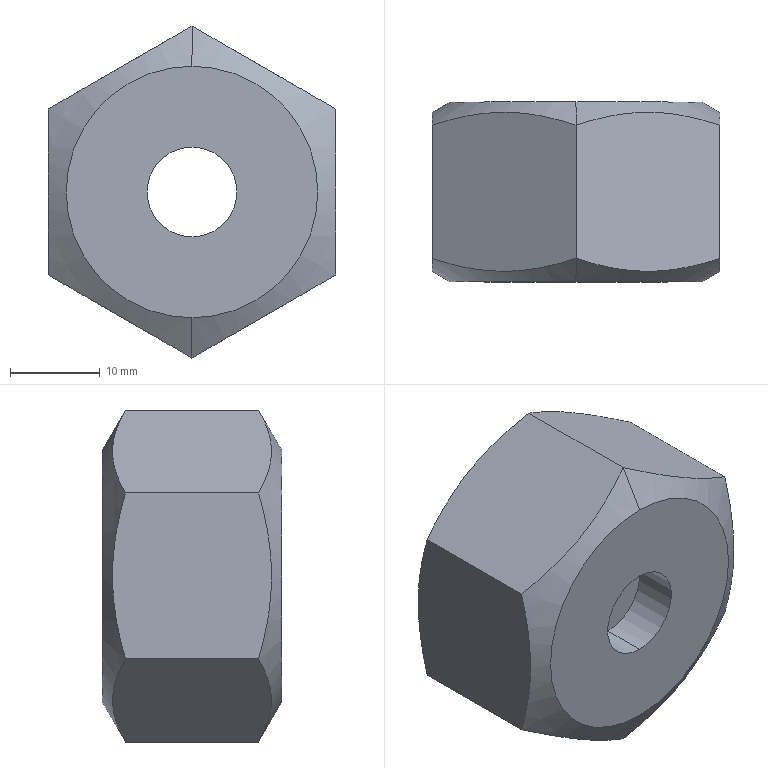Part | SolidWorks | features ICE 2, Extrusion 1, MirrorPattern 1, RevCut 1 | 1 solid | 20 faces | box 32 x 20 x 36.95 mm | volume 13532 mm3 | plane 10 | cylinder 6 | cone 4 | commonest cylinder face diameters 10 x4 28 x2
STEP:
#1=CARTESIAN_POINT('',(0.,-10.,14.));
#2=VERTEX_POINT('',#1);
#3=CARTESIAN_POINT('',(0.,-10.,-14.));
#4=VERTEX_POINT('',#3);
#5=CARTESIAN_POINT('',(0.,-10.,0.));
#6=DIRECTION('',(0.,-1.,0.));
#7=DIRECTION('',(0.,0.,-1.));
#8=AXIS2_PLACEMENT_3D('',#5,#6,#7);
#9=CIRCLE('',#8,14.);
#10=EDGE_CURVE('',#2,#4,#9,.T.);
#11=ORIENTED_EDGE('',*,*,#10,.F.);
#12=CARTESIAN_POINT('',(0.,-7.416,18.475));
#13=VERTEX_POINT('',#12);
#14=CARTESIAN_POINT('',(0.,-10.,14.));
#15=DIRECTION('',(0.,0.5,0.866));
#16=VECTOR('',#15,1000.);
#17=LINE('',#14,#16);
#18=EDGE_CURVE('',#2,#13,#17,.T.);
#19=ORIENTED_EDGE('',*,*,#18,.T.);
#20=CARTESIAN_POINT('',(-16.,-7.416,9.238));
#21=VERTEX_POINT('',#20);
#22=CARTESIAN_POINT('',(-16.,-7.416,9.238));
#23=CARTESIAN_POINT('',(-14.694,-7.852,9.992));
#24=CARTESIAN_POINT('',(-13.378,-8.211,10.751));
#25=CARTESIAN_POINT('',(-10.719,-8.708,12.287));
#26=CARTESIAN_POINT('',(-9.376,-8.844,13.062));
#27=CARTESIAN_POINT('',(-7.335,-8.846,14.24));
#28=CARTESIAN_POINT('',(-6.652,-8.812,14.635));
#29=CARTESIAN_POINT('',(-5.3,-8.682,15.415));
#30=CARTESIAN_POINT('',(-4.629,-8.585,15.803));
#31=CARTESIAN_POINT('',(-2.627,-8.212,16.959));
#32=CARTESIAN_POINT('',(-1.308,-7.852,17.72));
#33=CARTESIAN_POINT('',(0.,-7.416,18.475));
#34=B_SPLINE_CURVE_WITH_KNOTS('',3,(#22,#23,#24,#25,#26,#27,#28,#29,#30,#31,#32,#33),.UNSPECIFIED.,.F.,.F.,(4,2,2,2,2,4),(0.000000238,0.004665,0.00933,0.01166,0.01399,0.01866),.UNSPECIFIED.);
#35=EDGE_CURVE('',#21,#13,#34,.T.);
#36=ORIENTED_EDGE('',*,*,#35,.F.);
#37=CARTESIAN_POINT('',(-16.,-7.416,-9.238));
#38=VERTEX_POINT('',#37);
#39=CARTESIAN_POINT('',(-16.,-7.416,-9.238));
#40=CARTESIAN_POINT('',(-16.,-7.85,-7.733));
#41=CARTESIAN_POINT('',(-16.,-8.209,-6.216));
#42=CARTESIAN_POINT('',(-16.,-8.708,-3.141));
#43=CARTESIAN_POINT('',(-16.,-8.845,-1.584));
#44=CARTESIAN_POINT('',(-16.,-8.845,0.7894));
#45=CARTESIAN_POINT('',(-16.,-8.811,1.576));
#46=CARTESIAN_POINT('',(-16.,-8.68,3.136));
#47=CARTESIAN_POINT('',(-16.,-8.583,3.91));
#48=CARTESIAN_POINT('',(-16.,-8.209,6.217));
#49=CARTESIAN_POINT('',(-16.,-7.85,7.734));
#50=CARTESIAN_POINT('',(-16.,-7.416,9.238));
#51=B_SPLINE_CURVE_WITH_KNOTS('',3,(#39,#40,#41,#42,#43,#44,#45,#46,#47,#48,#49,#50),.UNSPECIFIED.,.F.,.F.,(4,2,2,2,2,4),(0.02027,0.02496,0.02966,0.03201,0.03436,0.03906),.UNSPECIFIED.);
#52=EDGE_CURVE('',#38,#21,#51,.T.);
#53=ORIENTED_EDGE('',*,*,#52,.F.);
#54=CARTESIAN_POINT('',(0.,-7.416,-18.475));
#55=VERTEX_POINT('',#54);
#56=CARTESIAN_POINT('',(0.,-7.416,-18.475));
#57=CARTESIAN_POINT('',(-1.306,-7.852,-17.721));
#58=CARTESIAN_POINT('',(-2.622,-8.211,-16.961));
#59=CARTESIAN_POINT('',(-5.281,-8.708,-15.426));
#60=CARTESIAN_POINT('',(-6.624,-8.844,-14.651));
#61=CARTESIAN_POINT('',(-8.665,-8.846,-13.473));
#62=CARTESIAN_POINT('',(-9.348,-8.812,-13.078));
#63=CARTESIAN_POINT('',(-10.7,-8.682,-12.298));
#64=CARTESIAN_POINT('',(-11.371,-8.585,-11.91));
#65=CARTESIAN_POINT('',(-13.373,-8.212,-10.754));
#66=CARTESIAN_POINT('',(-14.692,-7.852,-9.993));
#67=CARTESIAN_POINT('',(-16.,-7.416,-9.238));
#68=B_SPLINE_CURVE_WITH_KNOTS('',3,(#56,#57,#58,#59,#60,#61,#62,#63,#64,#65,#66,#67),.UNSPECIFIED.,.F.,.F.,(4,2,2,2,2,4),(0.000000238,0.004665,0.00933,0.01166,0.01399,0.01866),.UNSPECIFIED.);
#69=EDGE_CURVE('',#55,#38,#68,.T.);
#70=ORIENTED_EDGE('',*,*,#69,.F.);
#71=CARTESIAN_POINT('',(0.,-10.,-14.));
#72=DIRECTION('',(0.,0.5,-0.866));
#73=VECTOR('',#72,1000.);
#74=LINE('',#71,#73);
#75=EDGE_CURVE('',#4,#55,#74,.T.);
#76=ORIENTED_EDGE('',*,*,#75,.F.);
#77=EDGE_LOOP('',(#11,#19,#36,#53,#70,#76));
#78=FACE_OUTER_BOUND('',#77,.T.);
#79=CARTESIAN_POINT('',(0.,-10.,0.));
#80=DIRECTION('',(0.,1.,0.));
#81=DIRECTION('',(0.,0.,-1.));
#82=AXIS2_PLACEMENT_3D('',#79,#80,#81);
#83=CONICAL_SURFACE('',#82,14.,1.047);
#84=ADVANCED_FACE('',(#78),#83,.T.);
#85=CARTESIAN_POINT('',(0.,10.,-14.));
#86=VERTEX_POINT('',#85);
#87=CARTESIAN_POINT('',(0.,10.,14.));
#88=VERTEX_POINT('',#87);
#89=CARTESIAN_POINT('',(0.,10.,0.));
#90=DIRECTION('',(0.,-1.,0.));
#91=DIRECTION('',(0.,0.,-1.));
#92=AXIS2_PLACEMENT_3D('',#89,#90,#91);
#93=CIRCLE('',#92,14.);
#94=EDGE_CURVE('',#86,#88,#93,.T.);
#95=ORIENTED_EDGE('',*,*,#94,.T.);
#96=CARTESIAN_POINT('',(0.,7.416,18.475));
#97=VERTEX_POINT('',#96);
#98=CARTESIAN_POINT('',(0.,10.,14.));
#99=DIRECTION('',(0.,-0.5,0.866));
#100=VECTOR('',#99,1000.);
#101=LINE('',#98,#100);
#102=EDGE_CURVE('',#88,#97,#101,.T.);
#103=ORIENTED_EDGE('',*,*,#102,.T.);
#104=CARTESIAN_POINT('',(16.,7.416,9.238));
#105=VERTEX_POINT('',#104);
#106=CARTESIAN_POINT('',(16.,7.416,9.238));
#107=CARTESIAN_POINT('',(14.694,7.852,9.992));
#108=CARTESIAN_POINT('',(13.378,8.211,10.751));
#109=CARTESIAN_POINT('',(10.719,8.708,12.287));
#110=CARTESIAN_POINT('',(9.376,8.844,13.062));
#111=CARTESIAN_POINT('',(7.335,8.846,14.24));
#112=CARTESIAN_POINT('',(6.652,8.812,14.635));
#113=CARTESIAN_POINT('',(5.3,8.682,15.415));
#114=CARTESIAN_POINT('',(4.629,8.585,15.803));
#115=CARTESIAN_POINT('',(2.627,8.212,16.959));
#116=CARTESIAN_POINT('',(1.308,7.852,17.72));
#117=CARTESIAN_POINT('',(0.,7.416,18.475));
#118=B_SPLINE_CURVE_WITH_KNOTS('',3,(#106,#107,#108,#109,#110,#111,#112,#113,#114,#115,#116,#117),.UNSPECIFIED.,.F.,.F.,(4,2,2,2,2,4),(0.000000238,0.004665,0.00933,0.01166,0.01399,0.01866),.UNSPECIFIED.);
#119=EDGE_CURVE('',#105,#97,#118,.T.);
#120=ORIENTED_EDGE('',*,*,#119,.F.);
#121=CARTESIAN_POINT('',(16.,7.416,-9.238));
#122=VERTEX_POINT('',#121);
#123=CARTESIAN_POINT('',(16.,7.416,-9.238));
#124=CARTESIAN_POINT('',(16.,7.85,-7.733));
#125=CARTESIAN_POINT('',(16.,8.209,-6.216));
#126=CARTESIAN_POINT('',(16.,8.708,-3.141));
#127=CARTESIAN_POINT('',(16.,8.845,-1.584));
#128=CARTESIAN_POINT('',(16.,8.845,0.7894));
#129=CARTESIAN_POINT('',(16.,8.811,1.576));
#130=CARTESIAN_POINT('',(16.,8.68,3.136));
#131=CARTESIAN_POINT('',(16.,8.583,3.91));
#132=CARTESIAN_POINT('',(16.,8.209,6.217));
#133=CARTESIAN_POINT('',(16.,7.85,7.734));
#134=CARTESIAN_POINT('',(16.,7.416,9.238));
#135=B_SPLINE_CURVE_WITH_KNOTS('',3,(#123,#124,#125,#126,#127,#128,#129,#130,#131,#132,#133,#134),.UNSPECIFIED.,.F.,.F.,(4,2,2,2,2,4),(0.02027,0.02496,0.02966,0.03201,0.03436,0.03906),.UNSPECIFIED.);
#136=EDGE_CURVE('',#122,#105,#135,.T.);
#137=ORIENTED_EDGE('',*,*,#136,.F.);
#138=CARTESIAN_POINT('',(0.,7.416,-18.475));
#139=VERTEX_POINT('',#138);
#140=CARTESIAN_POINT('',(0.,7.416,-18.475));
#141=CARTESIAN_POINT('',(1.306,7.852,-17.721));
#142=CARTESIAN_POINT('',(2.622,8.211,-16.961));
#143=CARTESIAN_POINT('',(5.281,8.708,-15.426));
#144=CARTESIAN_POINT('',(6.624,8.844,-14.651));
#145=CARTESIAN_POINT('',(8.665,8.846,-13.473));
#146=CARTESIAN_POINT('',(9.348,8.812,-13.078));
#147=CARTESIAN_POINT('',(10.7,8.682,-12.298));
#148=CARTESIAN_POINT('',(11.371,8.585,-11.91));
#149=CARTESIAN_POINT('',(13.373,8.212,-10.754));
#150=CARTESIAN_POINT('',(14.692,7.852,-9.993));
#151=CARTESIAN_POINT('',(16.,7.416,-9.238));
#152=B_SPLINE_CURVE_WITH_KNOTS('',3,(#140,#141,#142,#143,#144,#145,#146,#147,#148,#149,#150,#151),.UNSPECIFIED.,.F.,.F.,(4,2,2,2,2,4),(0.000000238,0.004665,0.00933,0.01166,0.01399,0.01866),.UNSPECIFIED.);
#153=EDGE_CURVE('',#139,#122,#152,.T.);
#154=ORIENTED_EDGE('',*,*,#153,.F.);
#155=CARTESIAN_POINT('',(0.,10.,-14.));
#156=DIRECTION('',(0.,-0.5,-0.866));
#157=VECTOR('',#156,1000.);
#158=LINE('',#155,#157);
#159=EDGE_CURVE('',#86,#139,#158,.T.);
#160=ORIENTED_EDGE('',*,*,#159,.F.);
#161=EDGE_LOOP('',(#95,#103,#120,#137,#154,#160));
#162=FACE_OUTER_BOUND('',#161,.T.);
#163=CARTESIAN_POINT('',(0.,10.,0.));
#164=DIRECTION('',(0.,-1.,0.));
#165=DIRECTION('',(0.,0.,-1.));
#166=AXIS2_PLACEMENT_3D('',#163,#164,#165);
#167=CONICAL_SURFACE('',#166,14.,1.047);
#168=ADVANCED_FACE('',(#162),#167,.T.);
#169=CARTESIAN_POINT('',(0.,-1.,-14.));
#170=VERTEX_POINT('',#169);
#171=CARTESIAN_POINT('',(0.,-1.,14.));
#172=VERTEX_POINT('',#171);
#173=CARTESIAN_POINT('',(0.,-1.,0.));
#174=DIRECTION('',(0.,1.,0.));
#175=DIRECTION('',(0.,0.,1.));
#176=AXIS2_PLACEMENT_3D('',#173,#174,#175);
#177=CIRCLE('',#176,14.);
#178=EDGE_CURVE('',#170,#172,#177,.T.);
#179=ORIENTED_EDGE('',*,*,#178,.T.);
#180=CARTESIAN_POINT('',(0.,-5.,14.));
#181=VERTEX_POINT('',#180);
#182=CARTESIAN_POINT('',(0.,-1.,14.));
#183=DIRECTION('',(0.,-1.,0.));
#184=VECTOR('',#183,1000.);
#185=LINE('',#182,#184);
#186=EDGE_CURVE('',#172,#181,#185,.T.);
#187=ORIENTED_EDGE('',*,*,#186,.T.);
#188=CARTESIAN_POINT('',(0.,-5.,-14.));
#189=VERTEX_POINT('',#188);
#190=CARTESIAN_POINT('',(0.,-5.,0.));
#191=DIRECTION('',(0.,1.,0.));
#192=DIRECTION('',(0.,0.,1.));
#193=AXIS2_PLACEMENT_3D('',#190,#191,#192);
#194=CIRCLE('',#193,14.);
#195=EDGE_CURVE('',#189,#181,#194,.T.);
#196=ORIENTED_EDGE('',*,*,#195,.F.);
#197=CARTESIAN_POINT('',(0.,-1.,-14.));
#198=DIRECTION('',(0.,-1.,0.));
#199=VECTOR('',#198,1000.);
#200=LINE('',#197,#199);
#201=EDGE_CURVE('',#170,#189,#200,.T.);
#202=ORIENTED_EDGE('',*,*,#201,.F.);
#203=EDGE_LOOP('',(#179,#187,#196,#202));
#204=FACE_OUTER_BOUND('',#203,.T.);
#205=CARTESIAN_POINT('',(0.,-1.,0.));
#206=DIRECTION('',(0.,-1.,0.));
#207=DIRECTION('',(0.,0.,-1.));
#208=AXIS2_PLACEMENT_3D('',#205,#206,#207);
#209=CYLINDRICAL_SURFACE('',#208,14.);
#210=ADVANCED_FACE('',(#204),#209,.F.);
#211=CARTESIAN_POINT('',(0.,-1.,5.));
#212=VERTEX_POINT('',#211);
#213=CARTESIAN_POINT('',(0.,-1.,-5.));
#214=VERTEX_POINT('',#213);
#215=CARTESIAN_POINT('',(0.,-1.,0.));
#216=DIRECTION('',(0.,-1.,0.));
#217=DIRECTION('',(0.,0.,1.));
#218=AXIS2_PLACEMENT_3D('',#215,#216,#217);
#219=CIRCLE('',#218,5.);
#220=EDGE_CURVE('',#212,#214,#219,.T.);
#221=ORIENTED_EDGE('',*,*,#220,.T.);
#222=CARTESIAN_POINT('',(0.,10.,-5.));
#223=VERTEX_POINT('',#222);
#224=CARTESIAN_POINT('',(0.,-40.,-5.));
#225=DIRECTION('',(0.,1.,0.));
#226=VECTOR('',#225,1000.);
#227=LINE('',#224,#226);
#228=EDGE_CURVE('',#214,#223,#227,.T.);
#229=ORIENTED_EDGE('',*,*,#228,.T.);
#230=CARTESIAN_POINT('',(0.,10.,5.));
#231=VERTEX_POINT('',#230);
#232=CARTESIAN_POINT('',(0.,10.,0.));
#233=DIRECTION('',(0.,1.,0.));
#234=DIRECTION('',(0.,0.,1.));
#235=AXIS2_PLACEMENT_3D('',#232,#233,#234);
#236=CIRCLE('',#235,5.);
#237=EDGE_CURVE('',#223,#231,#236,.T.);
#238=ORIENTED_EDGE('',*,*,#237,.T.);
#239=CARTESIAN_POINT('',(0.,-40.,5.));
#240=DIRECTION('',(0.,1.,0.));
#241=VECTOR('',#240,1000.);
#242=LINE('',#239,#241);
#243=EDGE_CURVE('',#212,#231,#242,.T.);
#244=ORIENTED_EDGE('',*,*,#243,.F.);
#245=EDGE_LOOP('',(#221,#229,#238,#244));
#246=FACE_OUTER_BOUND('',#245,.T.);
#247=CARTESIAN_POINT('',(0.,-40.,0.));
#248=DIRECTION('',(0.,1.,0.));
#249=DIRECTION('',(0.,0.,1.));
#250=AXIS2_PLACEMENT_3D('',#247,#248,#249);
#251=CYLINDRICAL_SURFACE('',#250,5.);
#252=ADVANCED_FACE('',(#246),#251,.F.);
#253=CARTESIAN_POINT('',(0.,-10.,-5.));
#254=VERTEX_POINT('',#253);
#255=CARTESIAN_POINT('',(0.,-10.,5.));
#256=VERTEX_POINT('',#255);
#257=CARTESIAN_POINT('',(0.,-10.,0.));
#258=DIRECTION('',(0.,1.,0.));
#259=DIRECTION('',(0.,0.,1.));
#260=AXIS2_PLACEMENT_3D('',#257,#258,#259);
#261=CIRCLE('',#260,5.);
#262=EDGE_CURVE('',#254,#256,#261,.T.);
#263=ORIENTED_EDGE('',*,*,#262,.F.);
#264=CARTESIAN_POINT('',(0.,-5.,-5.));
#265=VERTEX_POINT('',#264);
#266=CARTESIAN_POINT('',(0.,-40.,-5.));
#267=DIRECTION('',(0.,1.,0.));
#268=VECTOR('',#267,1000.);
#269=LINE('',#266,#268);
#270=EDGE_CURVE('',#254,#265,#269,.T.);
#271=ORIENTED_EDGE('',*,*,#270,.T.);
#272=CARTESIAN_POINT('',(0.,-5.,5.));
#273=VERTEX_POINT('',#272);
#274=CARTESIAN_POINT('',(0.,-5.,0.));
#275=DIRECTION('',(0.,-1.,0.));
#276=DIRECTION('',(0.,0.,1.));
#277=AXIS2_PLACEMENT_3D('',#274,#275,#276);
#278=CIRCLE('',#277,5.);
#279=EDGE_CURVE('',#273,#265,#278,.T.);
#280=ORIENTED_EDGE('',*,*,#279,.F.);
#281=CARTESIAN_POINT('',(0.,-40.,5.));
#282=DIRECTION('',(0.,1.,0.));
#283=VECTOR('',#282,1000.);
#284=LINE('',#281,#283);
#285=EDGE_CURVE('',#256,#273,#284,.T.);
#286=ORIENTED_EDGE('',*,*,#285,.F.);
#287=EDGE_LOOP('',(#263,#271,#280,#286));
#288=FACE_OUTER_BOUND('',#287,.T.);
#289=CARTESIAN_POINT('',(0.,-40.,0.));
#290=DIRECTION('',(0.,1.,0.));
#291=DIRECTION('',(0.,0.,1.));
#292=AXIS2_PLACEMENT_3D('',#289,#290,#291);
#293=CYLINDRICAL_SURFACE('',#292,5.);
#294=ADVANCED_FACE('',(#288),#293,.F.);
#295=ORIENTED_EDGE('',*,*,#270,.F.);
#296=CARTESIAN_POINT('',(0.,-10.,0.));
#297=DIRECTION('',(0.,1.,0.));
#298=DIRECTION('',(0.,0.,1.));
#299=AXIS2_PLACEMENT_3D('',#296,#297,#298);
#300=CIRCLE('',#299,5.);
#301=EDGE_CURVE('',#256,#254,#300,.T.);
#302=ORIENTED_EDGE('',*,*,#301,.F.);
#303=ORIENTED_EDGE('',*,*,#285,.T.);
#304=CARTESIAN_POINT('',(0.,-5.,0.));
#305=DIRECTION('',(0.,-1.,0.));
#306=DIRECTION('',(0.,0.,1.));
#307=AXIS2_PLACEMENT_3D('',#304,#305,#306);
#308=CIRCLE('',#307,5.);
#309=EDGE_CURVE('',#265,#273,#308,.T.);
#310=ORIENTED_EDGE('',*,*,#309,.F.);
#311=EDGE_LOOP('',(#295,#302,#303,#310));
#312=FACE_OUTER_BOUND('',#311,.T.);
#313=CARTESIAN_POINT('',(0.,-40.,0.));
#314=DIRECTION('',(0.,1.,0.));
#315=DIRECTION('',(0.,0.,1.));
#316=AXIS2_PLACEMENT_3D('',#313,#314,#315);
#317=CYLINDRICAL_SURFACE('',#316,5.);
#318=ADVANCED_FACE('',(#312),#317,.F.);
#319=CARTESIAN_POINT('',(16.,-7.416,-9.238));
#320=VERTEX_POINT('',#319);
#321=CARTESIAN_POINT('',(16.,10.,-9.238));
#322=DIRECTION('',(0.,-1.,0.));
#323=VECTOR('',#322,1000.);
#324=LINE('',#321,#323);
#325=EDGE_CURVE('',#122,#320,#324,.T.);
#326=ORIENTED_EDGE('',*,*,#325,.T.);
#327=CARTESIAN_POINT('',(16.,-7.416,-9.238));
#328=CARTESIAN_POINT('',(14.694,-7.852,-9.992));
#329=CARTESIAN_POINT('',(13.378,-8.211,-10.751));
#330=CARTESIAN_POINT('',(10.719,-8.708,-12.287));
#331=CARTESIAN_POINT('',(9.376,-8.844,-13.062));
#332=CARTESIAN_POINT('',(7.335,-8.846,-14.24));
#333=CARTESIAN_POINT('',(6.652,-8.812,-14.635));
#334=CARTESIAN_POINT('',(5.3,-8.682,-15.415));
#335=CARTESIAN_POINT('',(4.629,-8.585,-15.803));
#336=CARTESIAN_POINT('',(2.627,-8.212,-16.959));
#337=CARTESIAN_POINT('',(1.308,-7.852,-17.72));
#338=CARTESIAN_POINT('',(0.,-7.416,-18.475));
#339=B_SPLINE_CURVE_WITH_KNOTS('',3,(#327,#328,#329,#330,#331,#332,#333,#334,#335,#336,#337,#338),.UNSPECIFIED.,.F.,.F.,(4,2,2,2,2,4),(0.000000238,0.004665,0.00933,0.01166,0.01399,0.01866),.UNSPECIFIED.);
#340=EDGE_CURVE('',#320,#55,#339,.T.);
#341=ORIENTED_EDGE('',*,*,#340,.T.);
#342=CARTESIAN_POINT('',(0.,10.,-18.475));
#343=DIRECTION('',(0.,-1.,0.));
#344=VECTOR('',#343,1000.);
#345=LINE('',#342,#344);
#346=EDGE_CURVE('',#139,#55,#345,.T.);
#347=ORIENTED_EDGE('',*,*,#346,.F.);
#348=ORIENTED_EDGE('',*,*,#153,.T.);
#349=EDGE_LOOP('',(#326,#341,#347,#348));
#350=FACE_OUTER_BOUND('',#349,.T.);
#351=CARTESIAN_POINT('',(16.,10.,-9.238));
#352=DIRECTION('',(-0.5,0.,0.866));
#353=DIRECTION('',(0.866,0.,0.5));
#354=AXIS2_PLACEMENT_3D('',#351,#352,#353);
#355=PLANE('',#354);
#356=ADVANCED_FACE('',(#350),#355,.F.);
#357=ORIENTED_EDGE('',*,*,#346,.T.);
#358=ORIENTED_EDGE('',*,*,#69,.T.);
#359=CARTESIAN_POINT('',(-16.,7.416,-9.238));
#360=VERTEX_POINT('',#359);
#361=CARTESIAN_POINT('',(-16.,10.,-9.238));
#362=DIRECTION('',(0.,-1.,0.));
#363=VECTOR('',#362,1000.);
#364=LINE('',#361,#363);
#365=EDGE_CURVE('',#360,#38,#364,.T.);
#366=ORIENTED_EDGE('',*,*,#365,.F.);
#367=CARTESIAN_POINT('',(-16.,7.416,-9.238));
#368=CARTESIAN_POINT('',(-14.694,7.852,-9.992));
#369=CARTESIAN_POINT('',(-13.378,8.211,-10.751));
#370=CARTESIAN_POINT('',(-10.719,8.708,-12.287));
#371=CARTESIAN_POINT('',(-9.376,8.844,-13.062));
#372=CARTESIAN_POINT('',(-7.335,8.846,-14.24));
#373=CARTESIAN_POINT('',(-6.652,8.812,-14.635));
#374=CARTESIAN_POINT('',(-5.3,8.682,-15.415));
#375=CARTESIAN_POINT('',(-4.629,8.585,-15.803));
#376=CARTESIAN_POINT('',(-2.627,8.212,-16.959));
#377=CARTESIAN_POINT('',(-1.308,7.852,-17.72));
#378=CARTESIAN_POINT('',(0.,7.416,-18.475));
#379=B_SPLINE_CURVE_WITH_KNOTS('',3,(#367,#368,#369,#370,#371,#372,#373,#374,#375,#376,#377,#378),.UNSPECIFIED.,.F.,.F.,(4,2,2,2,2,4),(0.000000238,0.004665,0.00933,0.01166,0.01399,0.01866),.UNSPECIFIED.);
#380=EDGE_CURVE('',#360,#139,#379,.T.);
#381=ORIENTED_EDGE('',*,*,#380,.T.);
#382=EDGE_LOOP('',(#357,#358,#366,#381));
#383=FACE_OUTER_BOUND('',#382,.T.);
#384=CARTESIAN_POINT('',(0.,10.,-18.475));
#385=DIRECTION('',(0.5,0.,0.866));
#386=DIRECTION('',(0.866,0.,-0.5));
#387=AXIS2_PLACEMENT_3D('',#384,#385,#386);
#388=PLANE('',#387);
#389=ADVANCED_FACE('',(#383),#388,.F.);
#390=ORIENTED_EDGE('',*,*,#365,.T.);
#391=ORIENTED_EDGE('',*,*,#52,.T.);
#392=CARTESIAN_POINT('',(-16.,7.416,9.238));
#393=VERTEX_POINT('',#392);
#394=CARTESIAN_POINT('',(-16.,10.,9.238));
#395=DIRECTION('',(0.,-1.,0.));
#396=VECTOR('',#395,1000.);
#397=LINE('',#394,#396);
#398=EDGE_CURVE('',#393,#21,#397,.T.);
#399=ORIENTED_EDGE('',*,*,#398,.F.);
#400=CARTESIAN_POINT('',(-16.,7.416,9.238));
#401=CARTESIAN_POINT('',(-16.,7.85,7.733));
#402=CARTESIAN_POINT('',(-16.,8.209,6.216));
#403=CARTESIAN_POINT('',(-16.,8.708,3.141));
#404=CARTESIAN_POINT('',(-16.,8.845,1.584));
#405=CARTESIAN_POINT('',(-16.,8.845,-0.7894));
#406=CARTESIAN_POINT('',(-16.,8.811,-1.576));
#407=CARTESIAN_POINT('',(-16.,8.68,-3.136));
#408=CARTESIAN_POINT('',(-16.,8.583,-3.91));
#409=CARTESIAN_POINT('',(-16.,8.209,-6.217));
#410=CARTESIAN_POINT('',(-16.,7.85,-7.734));
#411=CARTESIAN_POINT('',(-16.,7.416,-9.238));
#412=B_SPLINE_CURVE_WITH_KNOTS('',3,(#400,#401,#402,#403,#404,#405,#406,#407,#408,#409,#410,#411),.UNSPECIFIED.,.F.,.F.,(4,2,2,2,2,4),(0.02027,0.02496,0.02966,0.03201,0.03436,0.03906),.UNSPECIFIED.);
#413=EDGE_CURVE('',#393,#360,#412,.T.);
#414=ORIENTED_EDGE('',*,*,#413,.T.);
#415=EDGE_LOOP('',(#390,#391,#399,#414));
#416=FACE_OUTER_BOUND('',#415,.T.);
#417=CARTESIAN_POINT('',(-16.,10.,-9.238));
#418=DIRECTION('',(1.,0.,0.));
#419=DIRECTION('',(0.,0.,-1.));
#420=AXIS2_PLACEMENT_3D('',#417,#418,#419);
#421=PLANE('',#420);
#422=ADVANCED_FACE('',(#416),#421,.F.);
#423=ORIENTED_EDGE('',*,*,#398,.T.);
#424=ORIENTED_EDGE('',*,*,#35,.T.);
#425=CARTESIAN_POINT('',(0.,10.,18.475));
#426=DIRECTION('',(0.,-1.,0.));
#427=VECTOR('',#426,1000.);
#428=LINE('',#425,#427);
#429=EDGE_CURVE('',#97,#13,#428,.T.);
#430=ORIENTED_EDGE('',*,*,#429,.F.);
#431=CARTESIAN_POINT('',(0.,7.416,18.475));
#432=CARTESIAN_POINT('',(-1.306,7.852,17.721));
#433=CARTESIAN_POINT('',(-2.622,8.211,16.961));
#434=CARTESIAN_POINT('',(-5.281,8.708,15.426));
#435=CARTESIAN_POINT('',(-6.624,8.844,14.651));
#436=CARTESIAN_POINT('',(-8.665,8.846,13.473));
#437=CARTESIAN_POINT('',(-9.348,8.812,13.078));
#438=CARTESIAN_POINT('',(-10.7,8.682,12.298));
#439=CARTESIAN_POINT('',(-11.371,8.585,11.91));
#440=CARTESIAN_POINT('',(-13.373,8.212,10.754));
#441=CARTESIAN_POINT('',(-14.692,7.852,9.993));
#442=CARTESIAN_POINT('',(-16.,7.416,9.238));
#443=B_SPLINE_CURVE_WITH_KNOTS('',3,(#431,#432,#433,#434,#435,#436,#437,#438,#439,#440,#441,#442),.UNSPECIFIED.,.F.,.F.,(4,2,2,2,2,4),(0.000000238,0.004665,0.00933,0.01166,0.01399,0.01866),.UNSPECIFIED.);
#444=EDGE_CURVE('',#97,#393,#443,.T.);
#445=ORIENTED_EDGE('',*,*,#444,.T.);
#446=EDGE_LOOP('',(#423,#424,#430,#445));
#447=FACE_OUTER_BOUND('',#446,.T.);
#448=CARTESIAN_POINT('',(-16.,10.,9.238));
#449=DIRECTION('',(0.5,0.,-0.866));
#450=DIRECTION('',(-0.866,0.,-0.5));
#451=AXIS2_PLACEMENT_3D('',#448,#449,#450);
#452=PLANE('',#451);
#453=ADVANCED_FACE('',(#447),#452,.F.);
#454=ORIENTED_EDGE('',*,*,#429,.T.);
#455=CARTESIAN_POINT('',(16.,-7.416,9.238));
#456=VERTEX_POINT('',#455);
#457=CARTESIAN_POINT('',(0.,-7.416,18.475));
#458=CARTESIAN_POINT('',(1.306,-7.852,17.721));
#459=CARTESIAN_POINT('',(2.622,-8.211,16.961));
#460=CARTESIAN_POINT('',(5.281,-8.708,15.426));
#461=CARTESIAN_POINT('',(6.624,-8.844,14.651));
#462=CARTESIAN_POINT('',(8.665,-8.846,13.473));
#463=CARTESIAN_POINT('',(9.348,-8.812,13.078));
#464=CARTESIAN_POINT('',(10.7,-8.682,12.298));
#465=CARTESIAN_POINT('',(11.371,-8.585,11.91));
#466=CARTESIAN_POINT('',(13.373,-8.212,10.754));
#467=CARTESIAN_POINT('',(14.692,-7.852,9.993));
#468=CARTESIAN_POINT('',(16.,-7.416,9.238));
#469=B_SPLINE_CURVE_WITH_KNOTS('',3,(#457,#458,#459,#460,#461,#462,#463,#464,#465,#466,#467,#468),.UNSPECIFIED.,.F.,.F.,(4,2,2,2,2,4),(0.000000238,0.004665,0.00933,0.01166,0.01399,0.01866),.UNSPECIFIED.);
#470=EDGE_CURVE('',#13,#456,#469,.T.);
#471=ORIENTED_EDGE('',*,*,#470,.T.);
#472=CARTESIAN_POINT('',(16.,10.,9.238));
#473=DIRECTION('',(0.,-1.,0.));
#474=VECTOR('',#473,1000.);
#475=LINE('',#472,#474);
#476=EDGE_CURVE('',#105,#456,#475,.T.);
#477=ORIENTED_EDGE('',*,*,#476,.F.);
#478=ORIENTED_EDGE('',*,*,#119,.T.);
#479=EDGE_LOOP('',(#454,#471,#477,#478));
#480=FACE_OUTER_BOUND('',#479,.T.);
#481=CARTESIAN_POINT('',(0.,10.,18.475));
#482=DIRECTION('',(-0.5,0.,-0.866));
#483=DIRECTION('',(-0.866,0.,0.5));
#484=AXIS2_PLACEMENT_3D('',#481,#482,#483);
#485=PLANE('',#484);
#486=ADVANCED_FACE('',(#480),#485,.F.);
#487=ORIENTED_EDGE('',*,*,#476,.T.);
#488=CARTESIAN_POINT('',(16.,-7.416,9.238));
#489=CARTESIAN_POINT('',(16.,-7.85,7.733));
#490=CARTESIAN_POINT('',(16.,-8.209,6.216));
#491=CARTESIAN_POINT('',(16.,-8.708,3.141));
#492=CARTESIAN_POINT('',(16.,-8.845,1.584));
#493=CARTESIAN_POINT('',(16.,-8.845,-0.7894));
#494=CARTESIAN_POINT('',(16.,-8.811,-1.576));
#495=CARTESIAN_POINT('',(16.,-8.68,-3.136));
#496=CARTESIAN_POINT('',(16.,-8.583,-3.91));
#497=CARTESIAN_POINT('',(16.,-8.209,-6.217));
#498=CARTESIAN_POINT('',(16.,-7.85,-7.734));
#499=CARTESIAN_POINT('',(16.,-7.416,-9.238));
#500=B_SPLINE_CURVE_WITH_KNOTS('',3,(#488,#489,#490,#491,#492,#493,#494,#495,#496,#497,#498,#499),.UNSPECIFIED.,.F.,.F.,(4,2,2,2,2,4),(0.02027,0.02496,0.02966,0.03201,0.03436,0.03906),.UNSPECIFIED.);
#501=EDGE_CURVE('',#456,#320,#500,.T.);
#502=ORIENTED_EDGE('',*,*,#501,.T.);
#503=ORIENTED_EDGE('',*,*,#325,.F.);
#504=ORIENTED_EDGE('',*,*,#136,.T.);
#505=EDGE_LOOP('',(#487,#502,#503,#504));
#506=FACE_OUTER_BOUND('',#505,.T.);
#507=CARTESIAN_POINT('',(16.,10.,9.238));
#508=DIRECTION('',(-1.,0.,0.));
#509=DIRECTION('',(0.,0.,1.));
#510=AXIS2_PLACEMENT_3D('',#507,#508,#509);
#511=PLANE('',#510);
#512=ADVANCED_FACE('',(#506),#511,.F.);
#513=ORIENTED_EDGE('',*,*,#94,.F.);
#514=CARTESIAN_POINT('',(0.,10.,0.));
#515=DIRECTION('',(0.,-1.,0.));
#516=DIRECTION('',(0.,0.,-1.));
#517=AXIS2_PLACEMENT_3D('',#514,#515,#516);
#518=CIRCLE('',#517,14.);
#519=EDGE_CURVE('',#88,#86,#518,.T.);
#520=ORIENTED_EDGE('',*,*,#519,.F.);
#521=EDGE_LOOP('',(#513,#520));
#522=FACE_OUTER_BOUND('',#521,.T.);
#523=CARTESIAN_POINT('',(0.,10.,0.));
#524=DIRECTION('',(0.,1.,0.));
#525=DIRECTION('',(0.,0.,1.));
#526=AXIS2_PLACEMENT_3D('',#523,#524,#525);
#527=CIRCLE('',#526,5.);
#528=EDGE_CURVE('',#231,#223,#527,.T.);
#529=ORIENTED_EDGE('',*,*,#528,.F.);
#530=ORIENTED_EDGE('',*,*,#237,.F.);
#531=EDGE_LOOP('',(#529,#530));
#532=FACE_BOUND('',#531,.T.);
#533=CARTESIAN_POINT('',(0.,10.,0.));
#534=DIRECTION('',(0.,1.,0.));
#535=DIRECTION('',(0.,0.,1.));
#536=AXIS2_PLACEMENT_3D('',#533,#534,#535);
#537=PLANE('',#536);
#538=ADVANCED_FACE('',(#522,#532),#537,.T.);
#539=CARTESIAN_POINT('',(0.,-10.,0.));
#540=DIRECTION('',(0.,-1.,0.));
#541=DIRECTION('',(0.,0.,-1.));
#542=AXIS2_PLACEMENT_3D('',#539,#540,#541);
#543=CIRCLE('',#542,14.);
#544=EDGE_CURVE('',#4,#2,#543,.T.);
#545=ORIENTED_EDGE('',*,*,#544,.T.);
#546=ORIENTED_EDGE('',*,*,#10,.T.);
#547=EDGE_LOOP('',(#545,#546));
#548=FACE_OUTER_BOUND('',#547,.T.);
#549=ORIENTED_EDGE('',*,*,#301,.T.);
#550=ORIENTED_EDGE('',*,*,#262,.T.);
#551=EDGE_LOOP('',(#549,#550));
#552=FACE_BOUND('',#551,.T.);
#553=CARTESIAN_POINT('',(0.,-10.,0.));
#554=DIRECTION('',(0.,1.,0.));
#555=DIRECTION('',(0.,0.,1.));
#556=AXIS2_PLACEMENT_3D('',#553,#554,#555);
#557=PLANE('',#556);
#558=ADVANCED_FACE('',(#548,#552),#557,.F.);
#559=ORIENTED_EDGE('',*,*,#228,.F.);
#560=CARTESIAN_POINT('',(0.,-1.,0.));
#561=DIRECTION('',(0.,-1.,0.));
#562=DIRECTION('',(0.,0.,1.));
#563=AXIS2_PLACEMENT_3D('',#560,#561,#562);
#564=CIRCLE('',#563,5.);
#565=EDGE_CURVE('',#214,#212,#564,.T.);
#566=ORIENTED_EDGE('',*,*,#565,.T.);
#567=ORIENTED_EDGE('',*,*,#243,.T.);
#568=ORIENTED_EDGE('',*,*,#528,.T.);
#569=EDGE_LOOP('',(#559,#566,#567,#568));
#570=FACE_OUTER_BOUND('',#569,.T.);
#571=CARTESIAN_POINT('',(0.,-40.,0.));
#572=DIRECTION('',(0.,1.,0.));
#573=DIRECTION('',(0.,0.,1.));
#574=AXIS2_PLACEMENT_3D('',#571,#572,#573);
#575=CYLINDRICAL_SURFACE('',#574,5.);
#576=ADVANCED_FACE('',(#570),#575,.F.);
#577=ORIENTED_EDGE('',*,*,#178,.F.);
#578=CARTESIAN_POINT('',(0.,-1.,0.));
#579=DIRECTION('',(0.,1.,0.));
#580=DIRECTION('',(0.,0.,1.));
#581=AXIS2_PLACEMENT_3D('',#578,#579,#580);
#582=CIRCLE('',#581,14.);
#583=EDGE_CURVE('',#172,#170,#582,.T.);
#584=ORIENTED_EDGE('',*,*,#583,.F.);
#585=EDGE_LOOP('',(#577,#584));
#586=FACE_OUTER_BOUND('',#585,.T.);
#587=ORIENTED_EDGE('',*,*,#220,.F.);
#588=ORIENTED_EDGE('',*,*,#565,.F.);
#589=EDGE_LOOP('',(#587,#588));
#590=FACE_BOUND('',#589,.T.);
#591=CARTESIAN_POINT('',(0.,-1.,0.));
#592=DIRECTION('',(0.,1.,0.));
#593=DIRECTION('',(0.,0.,1.));
#594=AXIS2_PLACEMENT_3D('',#591,#592,#593);
#595=PLANE('',#594);
#596=ADVANCED_FACE('',(#586,#590),#595,.F.);
#597=ORIENTED_EDGE('',*,*,#195,.T.);
#598=CARTESIAN_POINT('',(0.,-5.,0.));
#599=DIRECTION('',(0.,1.,0.));
#600=DIRECTION('',(0.,0.,1.));
#601=AXIS2_PLACEMENT_3D('',#598,#599,#600);
#602=CIRCLE('',#601,14.);
#603=EDGE_CURVE('',#181,#189,#602,.T.);
#604=ORIENTED_EDGE('',*,*,#603,.T.);
#605=EDGE_LOOP('',(#597,#604));
#606=FACE_OUTER_BOUND('',#605,.T.);
#607=ORIENTED_EDGE('',*,*,#279,.T.);
#608=ORIENTED_EDGE('',*,*,#309,.T.);
#609=EDGE_LOOP('',(#607,#608));
#610=FACE_BOUND('',#609,.T.);
#611=CARTESIAN_POINT('',(0.,-5.,0.));
#612=DIRECTION('',(0.,1.,0.));
#613=DIRECTION('',(0.,0.,1.));
#614=AXIS2_PLACEMENT_3D('',#611,#612,#613);
#615=PLANE('',#614);
#616=ADVANCED_FACE('',(#606,#610),#615,.T.);
#617=ORIENTED_EDGE('',*,*,#186,.F.);
#618=ORIENTED_EDGE('',*,*,#583,.T.);
#619=ORIENTED_EDGE('',*,*,#201,.T.);
#620=ORIENTED_EDGE('',*,*,#603,.F.);
#621=EDGE_LOOP('',(#617,#618,#619,#620));
#622=FACE_OUTER_BOUND('',#621,.T.);
#623=CARTESIAN_POINT('',(0.,-1.,0.));
#624=DIRECTION('',(0.,-1.,0.));
#625=DIRECTION('',(0.,0.,-1.));
#626=AXIS2_PLACEMENT_3D('',#623,#624,#625);
#627=CYLINDRICAL_SURFACE('',#626,14.);
#628=ADVANCED_FACE('',(#622),#627,.F.);
#629=ORIENTED_EDGE('',*,*,#102,.F.);
#630=ORIENTED_EDGE('',*,*,#519,.T.);
#631=ORIENTED_EDGE('',*,*,#159,.T.);
#632=ORIENTED_EDGE('',*,*,#380,.F.);
#633=ORIENTED_EDGE('',*,*,#413,.F.);
#634=ORIENTED_EDGE('',*,*,#444,.F.);
#635=EDGE_LOOP('',(#629,#630,#631,#632,#633,#634));
#636=FACE_OUTER_BOUND('',#635,.T.);
#637=CARTESIAN_POINT('',(0.,10.,0.));
#638=DIRECTION('',(0.,-1.,0.));
#639=DIRECTION('',(0.,0.,-1.));
#640=AXIS2_PLACEMENT_3D('',#637,#638,#639);
#641=CONICAL_SURFACE('',#640,14.,1.047);
#642=ADVANCED_FACE('',(#636),#641,.T.);
#643=ORIENTED_EDGE('',*,*,#18,.F.);
#644=ORIENTED_EDGE('',*,*,#544,.F.);
#645=ORIENTED_EDGE('',*,*,#75,.T.);
#646=ORIENTED_EDGE('',*,*,#340,.F.);
#647=ORIENTED_EDGE('',*,*,#501,.F.);
#648=ORIENTED_EDGE('',*,*,#470,.F.);
#649=EDGE_LOOP('',(#643,#644,#645,#646,#647,#648));
#650=FACE_OUTER_BOUND('',#649,.T.);
#651=CARTESIAN_POINT('',(0.,-10.,0.));
#652=DIRECTION('',(0.,1.,0.));
#653=DIRECTION('',(0.,0.,-1.));
#654=AXIS2_PLACEMENT_3D('',#651,#652,#653);
#655=CONICAL_SURFACE('',#654,14.,1.047);
#656=ADVANCED_FACE('',(#650),#655,.T.);
#657=CLOSED_SHELL('',(#84,#168,#210,#252,#294,#318,#356,#389,#422,#453,#486,#512,#538,#558,#576,#596,#616,#628,#642,#656));
#658=MANIFOLD_SOLID_BREP('',#657);
#659=CARTESIAN_POINT('',(0.,0.,0.));
#660=DIRECTION('',(0.,0.,1.));
#661=DIRECTION('',(1.,0.,0.));
#662=AXIS2_PLACEMENT_3D('',#659,#660,#661);
#663=(LENGTH_UNIT()NAMED_UNIT(*)SI_UNIT(.MILLI.,.METRE.));
#664=UNCERTAINTY_MEASURE_WITH_UNIT(LENGTH_MEASURE(0.00001),#663,'','');
#665=(NAMED_UNIT(*)PLANE_ANGLE_UNIT()SI_UNIT($,.RADIAN.));
#666=(NAMED_UNIT(*)SI_UNIT($,.STERADIAN.)SOLID_ANGLE_UNIT());
#667=(GEOMETRIC_REPRESENTATION_CONTEXT(3)GLOBAL_UNCERTAINTY_ASSIGNED_CONTEXT((#664))GLOBAL_UNIT_ASSIGNED_CONTEXT((#663,#665,#666))REPRESENTATION_CONTEXT('',''));
#668=ADVANCED_BREP_SHAPE_REPRESENTATION('',(#658,#662),#667);